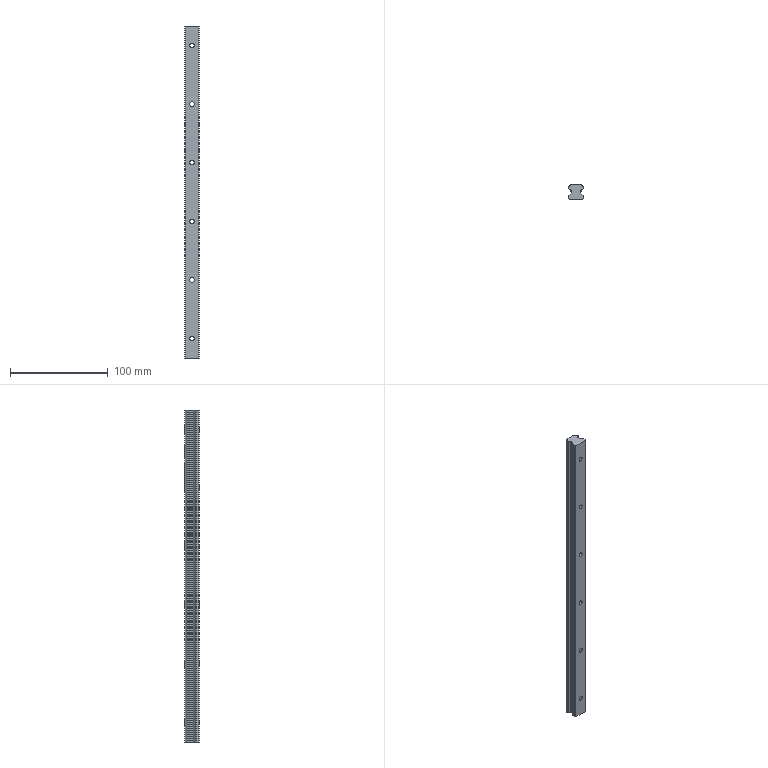Part | SolidWorks | features Extrusion 1, HoleWzd 1, ICE 1, LPattern 1 | 1 solid | 163 faces | box 15 x 15 x 340 mm | volume 62525 mm3 | plane 108 | cylinder 38 | spline 17 | commonest cylinder face diameters 4.5 x12 7.5 x12 0.8 x8 3.24 x4 2 x2